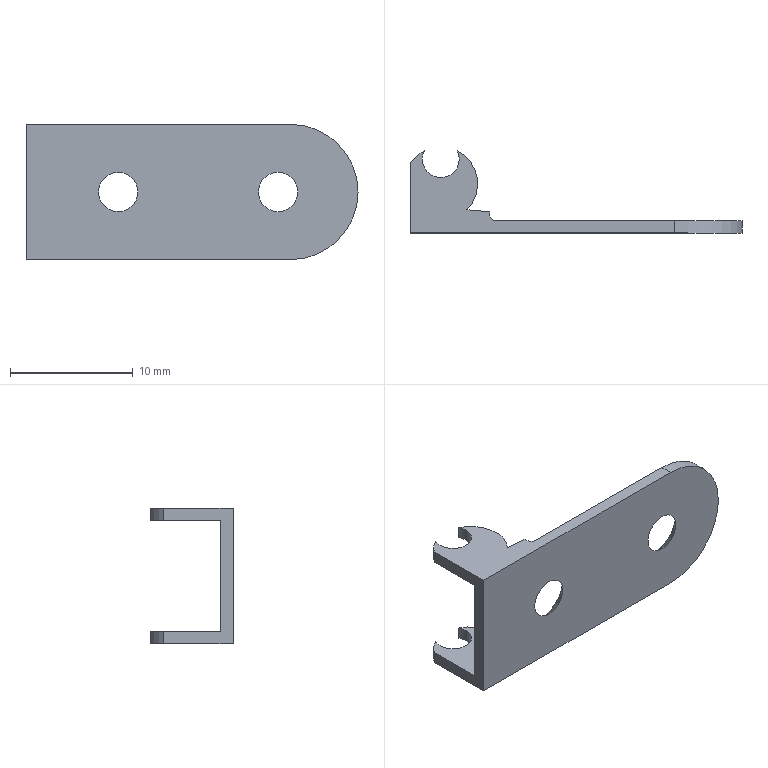Part | SolidWorks | features RefAxis 3, ICE 2, RevCut 2, 3DProfileFeature 1, Extrusion 1 | 1 solid | 28 faces | box 27 x 6.688 x 11 mm | volume 304.183 mm3 | cylinder 13 | plane 11 | cone 4 | commonest cylinder face diameters 3 x6 6 x4 1 x2 11 x1
STEP:
#1=CARTESIAN_POINT('',(20.5,0.,-1.6));
#2=VERTEX_POINT('',#1);
#3=CARTESIAN_POINT('',(20.5,0.,1.6));
#4=VERTEX_POINT('',#3);
#5=CARTESIAN_POINT('',(20.5,0.,0.));
#6=DIRECTION('',(0.,1.,0.));
#7=DIRECTION('',(0.,0.,1.));
#8=AXIS2_PLACEMENT_3D('',#5,#6,#7);
#9=CIRCLE('',#8,1.6);
#10=EDGE_CURVE('',#2,#4,#9,.T.);
#11=ORIENTED_EDGE('',*,*,#10,.F.);
#12=CARTESIAN_POINT('',(20.5,1.,-2.6));
#13=VERTEX_POINT('',#12);
#14=CARTESIAN_POINT('',(20.5,0.,-1.6));
#15=DIRECTION('',(0.,0.7071,-0.7071));
#16=VECTOR('',#15,1000.);
#17=LINE('',#14,#16);
#18=EDGE_CURVE('',#2,#13,#17,.T.);
#19=ORIENTED_EDGE('',*,*,#18,.T.);
#20=CARTESIAN_POINT('',(20.5,1.,2.6));
#21=VERTEX_POINT('',#20);
#22=CARTESIAN_POINT('',(20.5,1.,0.));
#23=DIRECTION('',(0.,1.,0.));
#24=DIRECTION('',(0.,0.,1.));
#25=AXIS2_PLACEMENT_3D('',#22,#23,#24);
#26=CIRCLE('',#25,2.6);
#27=EDGE_CURVE('',#13,#21,#26,.T.);
#28=ORIENTED_EDGE('',*,*,#27,.T.);
#29=CARTESIAN_POINT('',(20.5,0.,1.6));
#30=DIRECTION('',(0.,0.7071,0.7071));
#31=VECTOR('',#30,1000.);
#32=LINE('',#29,#31);
#33=EDGE_CURVE('',#4,#21,#32,.T.);
#34=ORIENTED_EDGE('',*,*,#33,.F.);
#35=EDGE_LOOP('',(#11,#19,#28,#34));
#36=FACE_OUTER_BOUND('',#35,.T.);
#37=CARTESIAN_POINT('',(20.5,0.,0.));
#38=DIRECTION('',(0.,1.,0.));
#39=DIRECTION('',(0.,0.,1.));
#40=AXIS2_PLACEMENT_3D('',#37,#38,#39);
#41=CONICAL_SURFACE('',#40,1.6,0.7854);
#42=ADVANCED_FACE('',(#36),#41,.F.);
#43=CARTESIAN_POINT('',(7.5,0.,-1.6));
#44=VERTEX_POINT('',#43);
#45=CARTESIAN_POINT('',(7.5,0.,1.6));
#46=VERTEX_POINT('',#45);
#47=CARTESIAN_POINT('',(7.5,0.,0.));
#48=DIRECTION('',(0.,1.,0.));
#49=DIRECTION('',(0.,0.,1.));
#50=AXIS2_PLACEMENT_3D('',#47,#48,#49);
#51=CIRCLE('',#50,1.6);
#52=EDGE_CURVE('',#44,#46,#51,.T.);
#53=ORIENTED_EDGE('',*,*,#52,.F.);
#54=CARTESIAN_POINT('',(7.5,1.,-2.6));
#55=VERTEX_POINT('',#54);
#56=CARTESIAN_POINT('',(7.5,0.,-1.6));
#57=DIRECTION('',(0.,0.7071,-0.7071));
#58=VECTOR('',#57,1000.);
#59=LINE('',#56,#58);
#60=EDGE_CURVE('',#44,#55,#59,.T.);
#61=ORIENTED_EDGE('',*,*,#60,.T.);
#62=CARTESIAN_POINT('',(7.5,1.,2.6));
#63=VERTEX_POINT('',#62);
#64=CARTESIAN_POINT('',(7.5,1.,0.));
#65=DIRECTION('',(0.,1.,0.));
#66=DIRECTION('',(0.,0.,1.));
#67=AXIS2_PLACEMENT_3D('',#64,#65,#66);
#68=CIRCLE('',#67,2.6);
#69=EDGE_CURVE('',#55,#63,#68,.T.);
#70=ORIENTED_EDGE('',*,*,#69,.T.);
#71=CARTESIAN_POINT('',(7.5,0.,1.6));
#72=DIRECTION('',(0.,0.7071,0.7071));
#73=VECTOR('',#72,1000.);
#74=LINE('',#71,#73);
#75=EDGE_CURVE('',#46,#63,#74,.T.);
#76=ORIENTED_EDGE('',*,*,#75,.F.);
#77=EDGE_LOOP('',(#53,#61,#70,#76));
#78=FACE_OUTER_BOUND('',#77,.T.);
#79=CARTESIAN_POINT('',(7.5,0.,0.));
#80=DIRECTION('',(0.,1.,0.));
#81=DIRECTION('',(0.,0.,1.));
#82=AXIS2_PLACEMENT_3D('',#79,#80,#81);
#83=CONICAL_SURFACE('',#82,1.6,0.7854);
#84=ADVANCED_FACE('',(#78),#83,.F.);
#85=CARTESIAN_POINT('',(4.,6.,-4.5));
#86=VERTEX_POINT('',#85);
#87=CARTESIAN_POINT('',(1.,6.,-4.5));
#88=VERTEX_POINT('',#87);
#89=CARTESIAN_POINT('',(2.5,6.,-4.5));
#90=DIRECTION('',(0.,0.,-1.));
#91=DIRECTION('',(1.,0.,0.));
#92=AXIS2_PLACEMENT_3D('',#89,#90,#91);
#93=CIRCLE('',#92,1.5);
#94=EDGE_CURVE('',#86,#88,#93,.T.);
#95=ORIENTED_EDGE('',*,*,#94,.F.);
#96=CARTESIAN_POINT('',(4.,6.,-5.5));
#97=VERTEX_POINT('',#96);
#98=CARTESIAN_POINT('',(4.,6.,5.5));
#99=DIRECTION('',(0.,0.,-1.));
#100=VECTOR('',#99,1000.);
#101=LINE('',#98,#100);
#102=EDGE_CURVE('',#86,#97,#101,.T.);
#103=ORIENTED_EDGE('',*,*,#102,.T.);
#104=CARTESIAN_POINT('',(1.,6.,-5.5));
#105=VERTEX_POINT('',#104);
#106=CARTESIAN_POINT('',(2.5,6.,-5.5));
#107=DIRECTION('',(0.,0.,-1.));
#108=DIRECTION('',(-1.,0.,0.));
#109=AXIS2_PLACEMENT_3D('',#106,#107,#108);
#110=CIRCLE('',#109,1.5);
#111=EDGE_CURVE('',#97,#105,#110,.T.);
#112=ORIENTED_EDGE('',*,*,#111,.T.);
#113=CARTESIAN_POINT('',(1.,6.,5.5));
#114=DIRECTION('',(0.,0.,-1.));
#115=VECTOR('',#114,1000.);
#116=LINE('',#113,#115);
#117=EDGE_CURVE('',#88,#105,#116,.T.);
#118=ORIENTED_EDGE('',*,*,#117,.F.);
#119=EDGE_LOOP('',(#95,#103,#112,#118));
#120=FACE_OUTER_BOUND('',#119,.T.);
#121=CARTESIAN_POINT('',(2.5,6.,5.5));
#122=DIRECTION('',(0.,0.,-1.));
#123=DIRECTION('',(-1.,0.,0.));
#124=AXIS2_PLACEMENT_3D('',#121,#122,#123);
#125=CYLINDRICAL_SURFACE('',#124,1.5);
#126=ADVANCED_FACE('',(#120),#125,.F.);
#127=CARTESIAN_POINT('',(1.167,6.688,-4.5));
#128=VERTEX_POINT('',#127);
#129=CARTESIAN_POINT('',(2.5,6.,-4.5));
#130=DIRECTION('',(0.,0.,-1.));
#131=DIRECTION('',(1.,0.,0.));
#132=AXIS2_PLACEMENT_3D('',#129,#130,#131);
#133=CIRCLE('',#132,1.5);
#134=EDGE_CURVE('',#88,#128,#133,.T.);
#135=ORIENTED_EDGE('',*,*,#134,.F.);
#136=ORIENTED_EDGE('',*,*,#117,.T.);
#137=CARTESIAN_POINT('',(1.167,6.688,-5.5));
#138=VERTEX_POINT('',#137);
#139=CARTESIAN_POINT('',(2.5,6.,-5.5));
#140=DIRECTION('',(0.,0.,-1.));
#141=DIRECTION('',(-1.,0.,0.));
#142=AXIS2_PLACEMENT_3D('',#139,#140,#141);
#143=CIRCLE('',#142,1.5);
#144=EDGE_CURVE('',#105,#138,#143,.T.);
#145=ORIENTED_EDGE('',*,*,#144,.T.);
#146=CARTESIAN_POINT('',(1.167,6.688,5.5));
#147=DIRECTION('',(0.,0.,-1.));
#148=VECTOR('',#147,1000.);
#149=LINE('',#146,#148);
#150=EDGE_CURVE('',#128,#138,#149,.T.);
#151=ORIENTED_EDGE('',*,*,#150,.F.);
#152=EDGE_LOOP('',(#135,#136,#145,#151));
#153=FACE_OUTER_BOUND('',#152,.T.);
#154=CARTESIAN_POINT('',(2.5,6.,5.5));
#155=DIRECTION('',(0.,0.,-1.));
#156=DIRECTION('',(-1.,0.,0.));
#157=AXIS2_PLACEMENT_3D('',#154,#155,#156);
#158=CYLINDRICAL_SURFACE('',#157,1.5);
#159=ADVANCED_FACE('',(#153),#158,.F.);
#160=CARTESIAN_POINT('',(4.,6.,5.5));
#161=VERTEX_POINT('',#160);
#162=CARTESIAN_POINT('',(1.,6.,5.5));
#163=VERTEX_POINT('',#162);
#164=CARTESIAN_POINT('',(2.5,6.,5.5));
#165=DIRECTION('',(0.,0.,-1.));
#166=DIRECTION('',(-1.,0.,0.));
#167=AXIS2_PLACEMENT_3D('',#164,#165,#166);
#168=CIRCLE('',#167,1.5);
#169=EDGE_CURVE('',#161,#163,#168,.T.);
#170=ORIENTED_EDGE('',*,*,#169,.F.);
#171=CARTESIAN_POINT('',(4.,6.,4.5));
#172=VERTEX_POINT('',#171);
#173=CARTESIAN_POINT('',(4.,6.,5.5));
#174=DIRECTION('',(0.,0.,-1.));
#175=VECTOR('',#174,1000.);
#176=LINE('',#173,#175);
#177=EDGE_CURVE('',#161,#172,#176,.T.);
#178=ORIENTED_EDGE('',*,*,#177,.T.);
#179=CARTESIAN_POINT('',(1.,6.,4.5));
#180=VERTEX_POINT('',#179);
#181=CARTESIAN_POINT('',(2.5,6.,4.5));
#182=DIRECTION('',(0.,0.,1.));
#183=DIRECTION('',(-1.,0.,0.));
#184=AXIS2_PLACEMENT_3D('',#181,#182,#183);
#185=CIRCLE('',#184,1.5);
#186=EDGE_CURVE('',#180,#172,#185,.T.);
#187=ORIENTED_EDGE('',*,*,#186,.F.);
#188=CARTESIAN_POINT('',(1.,6.,5.5));
#189=DIRECTION('',(0.,0.,-1.));
#190=VECTOR('',#189,1000.);
#191=LINE('',#188,#190);
#192=EDGE_CURVE('',#163,#180,#191,.T.);
#193=ORIENTED_EDGE('',*,*,#192,.F.);
#194=EDGE_LOOP('',(#170,#178,#187,#193));
#195=FACE_OUTER_BOUND('',#194,.T.);
#196=CARTESIAN_POINT('',(2.5,6.,5.5));
#197=DIRECTION('',(0.,0.,-1.));
#198=DIRECTION('',(-1.,0.,0.));
#199=AXIS2_PLACEMENT_3D('',#196,#197,#198);
#200=CYLINDRICAL_SURFACE('',#199,1.5);
#201=ADVANCED_FACE('',(#195),#200,.F.);
#202=CARTESIAN_POINT('',(1.167,6.688,5.5));
#203=VERTEX_POINT('',#202);
#204=CARTESIAN_POINT('',(2.5,6.,5.5));
#205=DIRECTION('',(0.,0.,-1.));
#206=DIRECTION('',(-1.,0.,0.));
#207=AXIS2_PLACEMENT_3D('',#204,#205,#206);
#208=CIRCLE('',#207,1.5);
#209=EDGE_CURVE('',#163,#203,#208,.T.);
#210=ORIENTED_EDGE('',*,*,#209,.F.);
#211=ORIENTED_EDGE('',*,*,#192,.T.);
#212=CARTESIAN_POINT('',(1.167,6.687,4.5));
#213=VERTEX_POINT('',#212);
#214=CARTESIAN_POINT('',(2.5,6.,4.5));
#215=DIRECTION('',(0.,0.,1.));
#216=DIRECTION('',(-1.,0.,0.));
#217=AXIS2_PLACEMENT_3D('',#214,#215,#216);
#218=CIRCLE('',#217,1.5);
#219=EDGE_CURVE('',#213,#180,#218,.T.);
#220=ORIENTED_EDGE('',*,*,#219,.F.);
#221=CARTESIAN_POINT('',(1.167,6.688,5.5));
#222=DIRECTION('',(0.,0.,-1.));
#223=VECTOR('',#222,1000.);
#224=LINE('',#221,#223);
#225=EDGE_CURVE('',#203,#213,#224,.T.);
#226=ORIENTED_EDGE('',*,*,#225,.F.);
#227=EDGE_LOOP('',(#210,#211,#220,#226));
#228=FACE_OUTER_BOUND('',#227,.T.);
#229=CARTESIAN_POINT('',(2.5,6.,5.5));
#230=DIRECTION('',(0.,0.,-1.));
#231=DIRECTION('',(-1.,0.,0.));
#232=AXIS2_PLACEMENT_3D('',#229,#230,#231);
#233=CYLINDRICAL_SURFACE('',#232,1.5);
#234=ADVANCED_FACE('',(#228),#233,.F.);
#235=CARTESIAN_POINT('',(7.5,0.,0.));
#236=DIRECTION('',(0.,1.,0.));
#237=DIRECTION('',(0.,0.,1.));
#238=AXIS2_PLACEMENT_3D('',#235,#236,#237);
#239=CIRCLE('',#238,1.6);
#240=EDGE_CURVE('',#46,#44,#239,.T.);
#241=ORIENTED_EDGE('',*,*,#240,.T.);
#242=ORIENTED_EDGE('',*,*,#52,.T.);
#243=EDGE_LOOP('',(#241,#242));
#244=FACE_BOUND('',#243,.T.);
#245=CARTESIAN_POINT('',(0.,0.,-5.5));
#246=VERTEX_POINT('',#245);
#247=CARTESIAN_POINT('',(21.5,0.,-5.5));
#248=VERTEX_POINT('',#247);
#249=CARTESIAN_POINT('',(0.,0.,-5.5));
#250=DIRECTION('',(1.,0.,0.));
#251=VECTOR('',#250,1000.);
#252=LINE('',#249,#251);
#253=EDGE_CURVE('',#246,#248,#252,.T.);
#254=ORIENTED_EDGE('',*,*,#253,.T.);
#255=CARTESIAN_POINT('',(21.5,0.,5.5));
#256=VERTEX_POINT('',#255);
#257=CARTESIAN_POINT('',(21.5,0.,0.));
#258=DIRECTION('',(0.,1.,0.));
#259=DIRECTION('',(0.,0.,1.));
#260=AXIS2_PLACEMENT_3D('',#257,#258,#259);
#261=CIRCLE('',#260,5.5);
#262=EDGE_CURVE('',#256,#248,#261,.T.);
#263=ORIENTED_EDGE('',*,*,#262,.F.);
#264=CARTESIAN_POINT('',(0.,0.,5.5));
#265=VERTEX_POINT('',#264);
#266=CARTESIAN_POINT('',(0.,0.,5.5));
#267=DIRECTION('',(1.,0.,0.));
#268=VECTOR('',#267,1000.);
#269=LINE('',#266,#268);
#270=EDGE_CURVE('',#265,#256,#269,.T.);
#271=ORIENTED_EDGE('',*,*,#270,.F.);
#272=CARTESIAN_POINT('',(0.,0.,5.5));
#273=DIRECTION('',(0.,0.,-1.));
#274=VECTOR('',#273,1000.);
#275=LINE('',#272,#274);
#276=EDGE_CURVE('',#265,#246,#275,.T.);
#277=ORIENTED_EDGE('',*,*,#276,.T.);
#278=EDGE_LOOP('',(#254,#263,#271,#277));
#279=FACE_OUTER_BOUND('',#278,.T.);
#280=CARTESIAN_POINT('',(20.5,0.,0.));
#281=DIRECTION('',(0.,1.,0.));
#282=DIRECTION('',(0.,0.,1.));
#283=AXIS2_PLACEMENT_3D('',#280,#281,#282);
#284=CIRCLE('',#283,1.6);
#285=EDGE_CURVE('',#4,#2,#284,.T.);
#286=ORIENTED_EDGE('',*,*,#285,.T.);
#287=ORIENTED_EDGE('',*,*,#10,.T.);
#288=EDGE_LOOP('',(#286,#287));
#289=FACE_BOUND('',#288,.T.);
#290=CARTESIAN_POINT('',(0.,0.,5.5));
#291=DIRECTION('',(0.,1.,0.));
#292=DIRECTION('',(0.,0.,1.));
#293=AXIS2_PLACEMENT_3D('',#290,#291,#292);
#294=PLANE('',#293);
#295=ADVANCED_FACE('',(#244,#279,#289),#294,.F.);
#296=CARTESIAN_POINT('',(7.5,1.,0.));
#297=DIRECTION('',(0.,1.,0.));
#298=DIRECTION('',(0.,0.,1.));
#299=AXIS2_PLACEMENT_3D('',#296,#297,#298);
#300=CIRCLE('',#299,2.6);
#301=EDGE_CURVE('',#63,#55,#300,.T.);
#302=ORIENTED_EDGE('',*,*,#301,.F.);
#303=ORIENTED_EDGE('',*,*,#69,.F.);
#304=EDGE_LOOP('',(#302,#303));
#305=FACE_BOUND('',#304,.T.);
#306=CARTESIAN_POINT('',(6.99,1.,-4.5));
#307=VERTEX_POINT('',#306);
#308=CARTESIAN_POINT('',(6.99,1.,-5.5));
#309=VERTEX_POINT('',#308);
#310=CARTESIAN_POINT('',(6.99,1.,5.5));
#311=DIRECTION('',(0.,0.,-1.));
#312=VECTOR('',#311,1000.);
#313=LINE('',#310,#312);
#314=EDGE_CURVE('',#307,#309,#313,.T.);
#315=ORIENTED_EDGE('',*,*,#314,.F.);
#316=CARTESIAN_POINT('',(0.,1.,-4.5));
#317=VERTEX_POINT('',#316);
#318=CARTESIAN_POINT('',(11.,1.,-4.5));
#319=DIRECTION('',(-1.,0.,0.));
#320=VECTOR('',#319,1000.);
#321=LINE('',#318,#320);
#322=EDGE_CURVE('',#307,#317,#321,.T.);
#323=ORIENTED_EDGE('',*,*,#322,.T.);
#324=CARTESIAN_POINT('',(0.,1.,4.5));
#325=VERTEX_POINT('',#324);
#326=CARTESIAN_POINT('',(0.,1.,4.5));
#327=DIRECTION('',(0.,0.,-1.));
#328=VECTOR('',#327,1000.);
#329=LINE('',#326,#328);
#330=EDGE_CURVE('',#325,#317,#329,.T.);
#331=ORIENTED_EDGE('',*,*,#330,.F.);
#332=CARTESIAN_POINT('',(6.99,1.,4.5));
#333=VERTEX_POINT('',#332);
#334=CARTESIAN_POINT('',(11.,1.,4.5));
#335=DIRECTION('',(-1.,0.,0.));
#336=VECTOR('',#335,1000.);
#337=LINE('',#334,#336);
#338=EDGE_CURVE('',#333,#325,#337,.T.);
#339=ORIENTED_EDGE('',*,*,#338,.F.);
#340=CARTESIAN_POINT('',(6.99,1.,5.5));
#341=VERTEX_POINT('',#340);
#342=CARTESIAN_POINT('',(6.99,1.,5.5));
#343=DIRECTION('',(0.,0.,-1.));
#344=VECTOR('',#343,1000.);
#345=LINE('',#342,#344);
#346=EDGE_CURVE('',#341,#333,#345,.T.);
#347=ORIENTED_EDGE('',*,*,#346,.F.);
#348=CARTESIAN_POINT('',(21.5,1.,5.5));
#349=VERTEX_POINT('',#348);
#350=CARTESIAN_POINT('',(27.,1.,5.5));
#351=DIRECTION('',(-1.,0.,0.));
#352=VECTOR('',#351,1000.);
#353=LINE('',#350,#352);
#354=EDGE_CURVE('',#349,#341,#353,.T.);
#355=ORIENTED_EDGE('',*,*,#354,.F.);
#356=CARTESIAN_POINT('',(21.5,1.,-5.5));
#357=VERTEX_POINT('',#356);
#358=CARTESIAN_POINT('',(21.5,1.,0.));
#359=DIRECTION('',(0.,1.,0.));
#360=DIRECTION('',(0.,0.,-1.));
#361=AXIS2_PLACEMENT_3D('',#358,#359,#360);
#362=CIRCLE('',#361,5.5);
#363=EDGE_CURVE('',#349,#357,#362,.T.);
#364=ORIENTED_EDGE('',*,*,#363,.T.);
#365=CARTESIAN_POINT('',(27.,1.,-5.5));
#366=DIRECTION('',(-1.,0.,0.));
#367=VECTOR('',#366,1000.);
#368=LINE('',#365,#367);
#369=EDGE_CURVE('',#357,#309,#368,.T.);
#370=ORIENTED_EDGE('',*,*,#369,.T.);
#371=EDGE_LOOP('',(#315,#323,#331,#339,#347,#355,#364,#370));
#372=FACE_OUTER_BOUND('',#371,.T.);
#373=CARTESIAN_POINT('',(20.5,1.,0.));
#374=DIRECTION('',(0.,1.,0.));
#375=DIRECTION('',(0.,0.,1.));
#376=AXIS2_PLACEMENT_3D('',#373,#374,#375);
#377=CIRCLE('',#376,2.6);
#378=EDGE_CURVE('',#21,#13,#377,.T.);
#379=ORIENTED_EDGE('',*,*,#378,.F.);
#380=ORIENTED_EDGE('',*,*,#27,.F.);
#381=EDGE_LOOP('',(#379,#380));
#382=FACE_BOUND('',#381,.T.);
#383=CARTESIAN_POINT('',(27.,1.,5.5));
#384=DIRECTION('',(0.,-1.,0.));
#385=DIRECTION('',(0.,0.,-1.));
#386=AXIS2_PLACEMENT_3D('',#383,#384,#385);
#387=PLANE('',#386);
#388=ADVANCED_FACE('',(#305,#372,#382),#387,.F.);
#389=CARTESIAN_POINT('',(0.,5.658,4.5));
#390=VERTEX_POINT('',#389);
#391=CARTESIAN_POINT('',(0.,11.,4.5));
#392=DIRECTION('',(0.,-1.,0.));
#393=VECTOR('',#392,1000.);
#394=LINE('',#391,#393);
#395=EDGE_CURVE('',#390,#325,#394,.T.);
#396=ORIENTED_EDGE('',*,*,#395,.T.);
#397=ORIENTED_EDGE('',*,*,#330,.T.);
#398=CARTESIAN_POINT('',(0.,5.658,-4.5));
#399=VERTEX_POINT('',#398);
#400=CARTESIAN_POINT('',(0.,1.,-4.5));
#401=DIRECTION('',(0.,1.,0.));
#402=VECTOR('',#401,1000.);
#403=LINE('',#400,#402);
#404=EDGE_CURVE('',#317,#399,#403,.T.);
#405=ORIENTED_EDGE('',*,*,#404,.T.);
#406=CARTESIAN_POINT('',(0.,5.658,-5.5));
#407=VERTEX_POINT('',#406);
#408=CARTESIAN_POINT('',(0.,5.658,5.5));
#409=DIRECTION('',(0.,0.,-1.));
#410=VECTOR('',#409,1000.);
#411=LINE('',#408,#410);
#412=EDGE_CURVE('',#399,#407,#411,.T.);
#413=ORIENTED_EDGE('',*,*,#412,.T.);
#414=CARTESIAN_POINT('',(0.,5.658,-5.5));
#415=DIRECTION('',(0.,-1.,0.));
#416=VECTOR('',#415,1000.);
#417=LINE('',#414,#416);
#418=EDGE_CURVE('',#407,#246,#417,.T.);
#419=ORIENTED_EDGE('',*,*,#418,.T.);
#420=ORIENTED_EDGE('',*,*,#276,.F.);
#421=CARTESIAN_POINT('',(0.,5.658,5.5));
#422=VERTEX_POINT('',#421);
#423=CARTESIAN_POINT('',(0.,5.658,5.5));
#424=DIRECTION('',(0.,-1.,0.));
#425=VECTOR('',#424,1000.);
#426=LINE('',#423,#425);
#427=EDGE_CURVE('',#422,#265,#426,.T.);
#428=ORIENTED_EDGE('',*,*,#427,.F.);
#429=CARTESIAN_POINT('',(0.,5.658,5.5));
#430=DIRECTION('',(0.,0.,-1.));
#431=VECTOR('',#430,1000.);
#432=LINE('',#429,#431);
#433=EDGE_CURVE('',#422,#390,#432,.T.);
#434=ORIENTED_EDGE('',*,*,#433,.T.);
#435=EDGE_LOOP('',(#396,#397,#405,#413,#419,#420,#428,#434));
#436=FACE_OUTER_BOUND('',#435,.T.);
#437=CARTESIAN_POINT('',(0.,5.658,5.5));
#438=DIRECTION('',(1.,0.,0.));
#439=DIRECTION('',(0.,0.,-1.));
#440=AXIS2_PLACEMENT_3D('',#437,#438,#439);
#441=PLANE('',#440);
#442=ADVANCED_FACE('',(#436),#441,.F.);
#443=CARTESIAN_POINT('',(6.49,1.5,4.5));
#444=VERTEX_POINT('',#443);
#445=CARTESIAN_POINT('',(6.99,1.5,4.5));
#446=DIRECTION('',(0.,0.,1.));
#447=DIRECTION('',(-1.,0.,0.));
#448=AXIS2_PLACEMENT_3D('',#445,#446,#447);
#449=CIRCLE('',#448,0.5);
#450=EDGE_CURVE('',#444,#333,#449,.T.);
#451=ORIENTED_EDGE('',*,*,#450,.F.);
#452=CARTESIAN_POINT('',(6.49,1.5,5.5));
#453=VERTEX_POINT('',#452);
#454=CARTESIAN_POINT('',(6.49,1.5,5.5));
#455=DIRECTION('',(0.,0.,-1.));
#456=VECTOR('',#455,1000.);
#457=LINE('',#454,#456);
#458=EDGE_CURVE('',#453,#444,#457,.T.);
#459=ORIENTED_EDGE('',*,*,#458,.F.);
#460=CARTESIAN_POINT('',(6.99,1.5,5.5));
#461=DIRECTION('',(0.,0.,-1.));
#462=DIRECTION('',(-1.,0.,0.));
#463=AXIS2_PLACEMENT_3D('',#460,#461,#462);
#464=CIRCLE('',#463,0.5);
#465=EDGE_CURVE('',#341,#453,#464,.T.);
#466=ORIENTED_EDGE('',*,*,#465,.F.);
#467=ORIENTED_EDGE('',*,*,#346,.T.);
#468=EDGE_LOOP('',(#451,#459,#466,#467));
#469=FACE_OUTER_BOUND('',#468,.T.);
#470=CARTESIAN_POINT('',(6.99,1.5,5.5));
#471=DIRECTION('',(0.,0.,-1.));
#472=DIRECTION('',(-1.,0.,0.));
#473=AXIS2_PLACEMENT_3D('',#470,#471,#472);
#474=CYLINDRICAL_SURFACE('',#473,0.5);
#475=ADVANCED_FACE('',(#469),#474,.F.);
#476=CARTESIAN_POINT('',(6.49,1.5,-4.5));
#477=VERTEX_POINT('',#476);
#478=CARTESIAN_POINT('',(6.99,1.5,-4.5));
#479=DIRECTION('',(0.,0.,-1.));
#480=DIRECTION('',(1.,0.,0.));
#481=AXIS2_PLACEMENT_3D('',#478,#479,#480);
#482=CIRCLE('',#481,0.5);
#483=EDGE_CURVE('',#307,#477,#482,.T.);
#484=ORIENTED_EDGE('',*,*,#483,.F.);
#485=ORIENTED_EDGE('',*,*,#314,.T.);
#486=CARTESIAN_POINT('',(6.49,1.5,-5.5));
#487=VERTEX_POINT('',#486);
#488=CARTESIAN_POINT('',(6.99,1.5,-5.5));
#489=DIRECTION('',(0.,0.,-1.));
#490=DIRECTION('',(-1.,0.,0.));
#491=AXIS2_PLACEMENT_3D('',#488,#489,#490);
#492=CIRCLE('',#491,0.5);
#493=EDGE_CURVE('',#309,#487,#492,.T.);
#494=ORIENTED_EDGE('',*,*,#493,.T.);
#495=CARTESIAN_POINT('',(6.49,1.5,5.5));
#496=DIRECTION('',(0.,0.,-1.));
#497=VECTOR('',#496,1000.);
#498=LINE('',#495,#497);
#499=EDGE_CURVE('',#477,#487,#498,.T.);
#500=ORIENTED_EDGE('',*,*,#499,.F.);
#501=EDGE_LOOP('',(#484,#485,#494,#500));
#502=FACE_OUTER_BOUND('',#501,.T.);
#503=CARTESIAN_POINT('',(6.99,1.5,5.5));
#504=DIRECTION('',(0.,0.,-1.));
#505=DIRECTION('',(-1.,0.,0.));
#506=AXIS2_PLACEMENT_3D('',#503,#504,#505);
#507=CYLINDRICAL_SURFACE('',#506,0.5);
#508=ADVANCED_FACE('',(#502),#507,.F.);
#509=CARTESIAN_POINT('',(6.49,1.725,4.5));
#510=VERTEX_POINT('',#509);
#511=CARTESIAN_POINT('',(6.49,1.5,4.5));
#512=DIRECTION('',(0.,-1.,0.));
#513=VECTOR('',#512,1000.);
#514=LINE('',#511,#513);
#515=EDGE_CURVE('',#510,#444,#514,.T.);
#516=ORIENTED_EDGE('',*,*,#515,.F.);
#517=CARTESIAN_POINT('',(6.49,1.725,5.5));
#518=VERTEX_POINT('',#517);
#519=CARTESIAN_POINT('',(6.49,1.725,5.5));
#520=DIRECTION('',(0.,0.,-1.));
#521=VECTOR('',#520,1000.);
#522=LINE('',#519,#521);
#523=EDGE_CURVE('',#518,#510,#522,.T.);
#524=ORIENTED_EDGE('',*,*,#523,.F.);
#525=CARTESIAN_POINT('',(6.49,1.5,5.5));
#526=DIRECTION('',(0.,1.,0.));
#527=VECTOR('',#526,1000.);
#528=LINE('',#525,#527);
#529=EDGE_CURVE('',#453,#518,#528,.T.);
#530=ORIENTED_EDGE('',*,*,#529,.F.);
#531=ORIENTED_EDGE('',*,*,#458,.T.);
#532=EDGE_LOOP('',(#516,#524,#530,#531));
#533=FACE_OUTER_BOUND('',#532,.T.);
#534=CARTESIAN_POINT('',(6.49,1.5,5.5));
#535=DIRECTION('',(-1.,0.,0.));
#536=DIRECTION('',(0.,0.,1.));
#537=AXIS2_PLACEMENT_3D('',#534,#535,#536);
#538=PLANE('',#537);
#539=ADVANCED_FACE('',(#533),#538,.F.);
#540=CARTESIAN_POINT('',(6.49,1.725,-4.5));
#541=VERTEX_POINT('',#540);
#542=CARTESIAN_POINT('',(6.49,1.5,-4.5));
#543=DIRECTION('',(0.,1.,0.));
#544=VECTOR('',#543,1000.);
#545=LINE('',#542,#544);
#546=EDGE_CURVE('',#477,#541,#545,.T.);
#547=ORIENTED_EDGE('',*,*,#546,.F.);
#548=ORIENTED_EDGE('',*,*,#499,.T.);
#549=CARTESIAN_POINT('',(6.49,1.725,-5.5));
#550=VERTEX_POINT('',#549);
#551=CARTESIAN_POINT('',(6.49,1.5,-5.5));
#552=DIRECTION('',(0.,1.,0.));
#553=VECTOR('',#552,1000.);
#554=LINE('',#551,#553);
#555=EDGE_CURVE('',#487,#550,#554,.T.);
#556=ORIENTED_EDGE('',*,*,#555,.T.);
#557=CARTESIAN_POINT('',(6.49,1.725,5.5));
#558=DIRECTION('',(0.,0.,-1.));
#559=VECTOR('',#558,1000.);
#560=LINE('',#557,#559);
#561=EDGE_CURVE('',#541,#550,#560,.T.);
#562=ORIENTED_EDGE('',*,*,#561,.F.);
#563=EDGE_LOOP('',(#547,#548,#556,#562));
#564=FACE_OUTER_BOUND('',#563,.T.);
#565=CARTESIAN_POINT('',(6.49,1.5,5.5));
#566=DIRECTION('',(-1.,0.,0.));
#567=DIRECTION('',(0.,0.,1.));
#568=AXIS2_PLACEMENT_3D('',#565,#566,#567);
#569=PLANE('',#568);
#570=ADVANCED_FACE('',(#564),#569,.F.);
#571=CARTESIAN_POINT('',(4.63,1.887,4.5));
#572=VERTEX_POINT('',#571);
#573=CARTESIAN_POINT('',(6.49,1.725,4.5));
#574=DIRECTION('',(0.9962,-0.08716,0.));
#575=VECTOR('',#574,1000.);
#576=LINE('',#573,#575);
#577=EDGE_CURVE('',#572,#510,#576,.T.);
#578=ORIENTED_EDGE('',*,*,#577,.F.);
#579=CARTESIAN_POINT('',(4.63,1.887,5.5));
#580=VERTEX_POINT('',#579);
#581=CARTESIAN_POINT('',(4.63,1.887,5.5));
#582=DIRECTION('',(0.,0.,-1.));
#583=VECTOR('',#582,1000.);
#584=LINE('',#581,#583);
#585=EDGE_CURVE('',#580,#572,#584,.T.);
#586=ORIENTED_EDGE('',*,*,#585,.F.);
#587=CARTESIAN_POINT('',(6.49,1.725,5.5));
#588=DIRECTION('',(-0.9962,0.08716,0.));
#589=VECTOR('',#588,1000.);
#590=LINE('',#587,#589);
#591=EDGE_CURVE('',#518,#580,#590,.T.);
#592=ORIENTED_EDGE('',*,*,#591,.F.);
#593=ORIENTED_EDGE('',*,*,#523,.T.);
#594=EDGE_LOOP('',(#578,#586,#592,#593));
#595=FACE_OUTER_BOUND('',#594,.T.);
#596=CARTESIAN_POINT('',(6.49,1.725,5.5));
#597=DIRECTION('',(-0.08716,-0.9962,0.));
#598=DIRECTION('',(0.9962,-0.08716,0.));
#599=AXIS2_PLACEMENT_3D('',#596,#597,#598);
#600=PLANE('',#599);
#601=ADVANCED_FACE('',(#595),#600,.F.);
#602=CARTESIAN_POINT('',(4.63,1.887,-4.5));
#603=VERTEX_POINT('',#602);
#604=CARTESIAN_POINT('',(6.49,1.725,-4.5));
#605=DIRECTION('',(-0.9962,0.08716,0.));
#606=VECTOR('',#605,1000.);
#607=LINE('',#604,#606);
#608=EDGE_CURVE('',#541,#603,#607,.T.);
#609=ORIENTED_EDGE('',*,*,#608,.F.);
#610=ORIENTED_EDGE('',*,*,#561,.T.);
#611=CARTESIAN_POINT('',(4.63,1.887,-5.5));
#612=VERTEX_POINT('',#611);
#613=CARTESIAN_POINT('',(6.49,1.725,-5.5));
#614=DIRECTION('',(-0.9962,0.08716,0.));
#615=VECTOR('',#614,1000.);
#616=LINE('',#613,#615);
#617=EDGE_CURVE('',#550,#612,#616,.T.);
#618=ORIENTED_EDGE('',*,*,#617,.T.);
#619=CARTESIAN_POINT('',(4.63,1.887,5.5));
#620=DIRECTION('',(0.,0.,-1.));
#621=VECTOR('',#620,1000.);
#622=LINE('',#619,#621);
#623=EDGE_CURVE('',#603,#612,#622,.T.);
#624=ORIENTED_EDGE('',*,*,#623,.F.);
#625=EDGE_LOOP('',(#609,#610,#618,#624));
#626=FACE_OUTER_BOUND('',#625,.T.);
#627=CARTESIAN_POINT('',(6.49,1.725,5.5));
#628=DIRECTION('',(-0.08716,-0.9962,0.));
#629=DIRECTION('',(0.9962,-0.08716,0.));
#630=AXIS2_PLACEMENT_3D('',#627,#628,#629);
#631=PLANE('',#630);
#632=ADVANCED_FACE('',(#626),#631,.F.);
#633=CARTESIAN_POINT('',(3.833,6.687,4.5));
#634=VERTEX_POINT('',#633);
#635=CARTESIAN_POINT('',(2.5,4.,4.5));
#636=DIRECTION('',(0.,0.,-1.));
#637=DIRECTION('',(-1.,0.,0.));
#638=AXIS2_PLACEMENT_3D('',#635,#636,#637);
#639=CIRCLE('',#638,3.);
#640=EDGE_CURVE('',#634,#572,#639,.T.);
#641=ORIENTED_EDGE('',*,*,#640,.F.);
#642=CARTESIAN_POINT('',(3.833,6.687,5.5));
#643=VERTEX_POINT('',#642);
#644=CARTESIAN_POINT('',(3.833,6.687,5.5));
#645=DIRECTION('',(0.,0.,-1.));
#646=VECTOR('',#645,1000.);
#647=LINE('',#644,#646);
#648=EDGE_CURVE('',#643,#634,#647,.T.);
#649=ORIENTED_EDGE('',*,*,#648,.F.);
#650=CARTESIAN_POINT('',(2.5,4.,5.5));
#651=DIRECTION('',(0.,0.,1.));
#652=DIRECTION('',(1.,0.,0.));
#653=AXIS2_PLACEMENT_3D('',#650,#651,#652);
#654=CIRCLE('',#653,3.);
#655=EDGE_CURVE('',#580,#643,#654,.T.);
#656=ORIENTED_EDGE('',*,*,#655,.F.);
#657=ORIENTED_EDGE('',*,*,#585,.T.);
#658=EDGE_LOOP('',(#641,#649,#656,#657));
#659=FACE_OUTER_BOUND('',#658,.T.);
#660=CARTESIAN_POINT('',(2.5,4.,5.5));
#661=DIRECTION('',(0.,0.,-1.));
#662=DIRECTION('',(-1.,0.,0.));
#663=AXIS2_PLACEMENT_3D('',#660,#661,#662);
#664=CYLINDRICAL_SURFACE('',#663,3.);
#665=ADVANCED_FACE('',(#659),#664,.T.);
#666=CARTESIAN_POINT('',(3.833,6.687,-4.5));
#667=VERTEX_POINT('',#666);
#668=CARTESIAN_POINT('',(2.5,4.,-4.5));
#669=DIRECTION('',(0.,0.,1.));
#670=DIRECTION('',(1.,0.,0.));
#671=AXIS2_PLACEMENT_3D('',#668,#669,#670);
#672=CIRCLE('',#671,3.);
#673=EDGE_CURVE('',#603,#667,#672,.T.);
#674=ORIENTED_EDGE('',*,*,#673,.F.);
#675=ORIENTED_EDGE('',*,*,#623,.T.);
#676=CARTESIAN_POINT('',(3.833,6.687,-5.5));
#677=VERTEX_POINT('',#676);
#678=CARTESIAN_POINT('',(2.5,4.,-5.5));
#679=DIRECTION('',(0.,0.,1.));
#680=DIRECTION('',(1.,0.,0.));
#681=AXIS2_PLACEMENT_3D('',#678,#679,#680);
#682=CIRCLE('',#681,3.);
#683=EDGE_CURVE('',#612,#677,#682,.T.);
#684=ORIENTED_EDGE('',*,*,#683,.T.);
#685=CARTESIAN_POINT('',(3.833,6.687,5.5));
#686=DIRECTION('',(0.,0.,-1.));
#687=VECTOR('',#686,1000.);
#688=LINE('',#685,#687);
#689=EDGE_CURVE('',#667,#677,#688,.T.);
#690=ORIENTED_EDGE('',*,*,#689,.F.);
#691=EDGE_LOOP('',(#674,#675,#684,#690));
#692=FACE_OUTER_BOUND('',#691,.T.);
#693=CARTESIAN_POINT('',(2.5,4.,5.5));
#694=DIRECTION('',(0.,0.,-1.));
#695=DIRECTION('',(-1.,0.,0.));
#696=AXIS2_PLACEMENT_3D('',#693,#694,#695);
#697=CYLINDRICAL_SURFACE('',#696,3.);
#698=ADVANCED_FACE('',(#692),#697,.T.);
#699=ORIENTED_EDGE('',*,*,#177,.F.);
#700=CARTESIAN_POINT('',(2.5,6.,5.5));
#701=DIRECTION('',(0.,0.,-1.));
#702=DIRECTION('',(-1.,0.,0.));
#703=AXIS2_PLACEMENT_3D('',#700,#701,#702);
#704=CIRCLE('',#703,1.5);
#705=EDGE_CURVE('',#643,#161,#704,.T.);
#706=ORIENTED_EDGE('',*,*,#705,.F.);
#707=ORIENTED_EDGE('',*,*,#648,.T.);
#708=CARTESIAN_POINT('',(2.5,6.,4.5));
#709=DIRECTION('',(0.,0.,1.));
#710=DIRECTION('',(-1.,0.,0.));
#711=AXIS2_PLACEMENT_3D('',#708,#709,#710);
#712=CIRCLE('',#711,1.5);
#713=EDGE_CURVE('',#172,#634,#712,.T.);
#714=ORIENTED_EDGE('',*,*,#713,.F.);
#715=EDGE_LOOP('',(#699,#706,#707,#714));
#716=FACE_OUTER_BOUND('',#715,.T.);
#717=CARTESIAN_POINT('',(2.5,6.,5.5));
#718=DIRECTION('',(0.,0.,-1.));
#719=DIRECTION('',(-1.,0.,0.));
#720=AXIS2_PLACEMENT_3D('',#717,#718,#719);
#721=CYLINDRICAL_SURFACE('',#720,1.5);
#722=ADVANCED_FACE('',(#716),#721,.F.);
#723=ORIENTED_EDGE('',*,*,#102,.F.);
#724=CARTESIAN_POINT('',(2.5,6.,-4.5));
#725=DIRECTION('',(0.,0.,-1.));
#726=DIRECTION('',(1.,0.,0.));
#727=AXIS2_PLACEMENT_3D('',#724,#725,#726);
#728=CIRCLE('',#727,1.5);
#729=EDGE_CURVE('',#667,#86,#728,.T.);
#730=ORIENTED_EDGE('',*,*,#729,.F.);
#731=ORIENTED_EDGE('',*,*,#689,.T.);
#732=CARTESIAN_POINT('',(2.5,6.,-5.5));
#733=DIRECTION('',(0.,0.,-1.));
#734=DIRECTION('',(-1.,0.,0.));
#735=AXIS2_PLACEMENT_3D('',#732,#733,#734);
#736=CIRCLE('',#735,1.5);
#737=EDGE_CURVE('',#677,#97,#736,.T.);
#738=ORIENTED_EDGE('',*,*,#737,.T.);
#739=EDGE_LOOP('',(#723,#730,#731,#738));
#740=FACE_OUTER_BOUND('',#739,.T.);
#741=CARTESIAN_POINT('',(2.5,6.,5.5));
#742=DIRECTION('',(0.,0.,-1.));
#743=DIRECTION('',(-1.,0.,0.));
#744=AXIS2_PLACEMENT_3D('',#741,#742,#743);
#745=CYLINDRICAL_SURFACE('',#744,1.5);
#746=ADVANCED_FACE('',(#740),#745,.F.);
#747=CARTESIAN_POINT('',(2.5,4.,4.5));
#748=DIRECTION('',(0.,0.,-1.));
#749=DIRECTION('',(-1.,0.,0.));
#750=AXIS2_PLACEMENT_3D('',#747,#748,#749);
#751=CIRCLE('',#750,3.);
#752=EDGE_CURVE('',#390,#213,#751,.T.);
#753=ORIENTED_EDGE('',*,*,#752,.F.);
#754=ORIENTED_EDGE('',*,*,#433,.F.);
#755=CARTESIAN_POINT('',(2.5,4.,5.5));
#756=DIRECTION('',(0.,0.,1.));
#757=DIRECTION('',(1.,0.,0.));
#758=AXIS2_PLACEMENT_3D('',#755,#756,#757);
#759=CIRCLE('',#758,3.);
#760=EDGE_CURVE('',#203,#422,#759,.T.);
#761=ORIENTED_EDGE('',*,*,#760,.F.);
#762=ORIENTED_EDGE('',*,*,#225,.T.);
#763=EDGE_LOOP('',(#753,#754,#761,#762));
#764=FACE_OUTER_BOUND('',#763,.T.);
#765=CARTESIAN_POINT('',(2.5,4.,5.5));
#766=DIRECTION('',(0.,0.,-1.));
#767=DIRECTION('',(-1.,0.,0.));
#768=AXIS2_PLACEMENT_3D('',#765,#766,#767);
#769=CYLINDRICAL_SURFACE('',#768,3.);
#770=ADVANCED_FACE('',(#764),#769,.T.);
#771=CARTESIAN_POINT('',(2.5,4.,-4.5));
#772=DIRECTION('',(0.,0.,1.));
#773=DIRECTION('',(1.,0.,0.));
#774=AXIS2_PLACEMENT_3D('',#771,#772,#773);
#775=CIRCLE('',#774,3.);
#776=EDGE_CURVE('',#128,#399,#775,.T.);
#777=ORIENTED_EDGE('',*,*,#776,.F.);
#778=ORIENTED_EDGE('',*,*,#150,.T.);
#779=CARTESIAN_POINT('',(2.5,4.,-5.5));
#780=DIRECTION('',(0.,0.,1.));
#781=DIRECTION('',(1.,0.,0.));
#782=AXIS2_PLACEMENT_3D('',#779,#780,#781);
#783=CIRCLE('',#782,3.);
#784=EDGE_CURVE('',#138,#407,#783,.T.);
#785=ORIENTED_EDGE('',*,*,#784,.T.);
#786=ORIENTED_EDGE('',*,*,#412,.F.);
#787=EDGE_LOOP('',(#777,#778,#785,#786));
#788=FACE_OUTER_BOUND('',#787,.T.);
#789=CARTESIAN_POINT('',(2.5,4.,5.5));
#790=DIRECTION('',(0.,0.,-1.));
#791=DIRECTION('',(-1.,0.,0.));
#792=AXIS2_PLACEMENT_3D('',#789,#790,#791);
#793=CYLINDRICAL_SURFACE('',#792,3.);
#794=ADVANCED_FACE('',(#788),#793,.T.);
#795=ORIENTED_EDGE('',*,*,#270,.T.);
#796=CARTESIAN_POINT('',(21.5,11.,5.5));
#797=DIRECTION('',(0.,-1.,0.));
#798=VECTOR('',#797,1000.);
#799=LINE('',#796,#798);
#800=EDGE_CURVE('',#349,#256,#799,.T.);
#801=ORIENTED_EDGE('',*,*,#800,.F.);
#802=ORIENTED_EDGE('',*,*,#354,.T.);
#803=ORIENTED_EDGE('',*,*,#465,.T.);
#804=ORIENTED_EDGE('',*,*,#529,.T.);
#805=ORIENTED_EDGE('',*,*,#591,.T.);
#806=ORIENTED_EDGE('',*,*,#655,.T.);
#807=ORIENTED_EDGE('',*,*,#705,.T.);
#808=ORIENTED_EDGE('',*,*,#169,.T.);
#809=ORIENTED_EDGE('',*,*,#209,.T.);
#810=ORIENTED_EDGE('',*,*,#760,.T.);
#811=ORIENTED_EDGE('',*,*,#427,.T.);
#812=EDGE_LOOP('',(#795,#801,#802,#803,#804,#805,#806,#807,#808,#809,#810,#811));
#813=FACE_OUTER_BOUND('',#812,.T.);
#814=CARTESIAN_POINT('',(6.99,1.5,5.5));
#815=DIRECTION('',(0.,0.,-1.));
#816=DIRECTION('',(-1.,0.,0.));
#817=AXIS2_PLACEMENT_3D('',#814,#815,#816);
#818=PLANE('',#817);
#819=ADVANCED_FACE('',(#813),#818,.F.);
#820=CARTESIAN_POINT('',(21.5,11.,-5.5));
#821=DIRECTION('',(0.,1.,0.));
#822=VECTOR('',#821,1000.);
#823=LINE('',#820,#822);
#824=EDGE_CURVE('',#248,#357,#823,.T.);
#825=ORIENTED_EDGE('',*,*,#824,.F.);
#826=ORIENTED_EDGE('',*,*,#253,.F.);
#827=ORIENTED_EDGE('',*,*,#418,.F.);
#828=ORIENTED_EDGE('',*,*,#784,.F.);
#829=ORIENTED_EDGE('',*,*,#144,.F.);
#830=ORIENTED_EDGE('',*,*,#111,.F.);
#831=ORIENTED_EDGE('',*,*,#737,.F.);
#832=ORIENTED_EDGE('',*,*,#683,.F.);
#833=ORIENTED_EDGE('',*,*,#617,.F.);
#834=ORIENTED_EDGE('',*,*,#555,.F.);
#835=ORIENTED_EDGE('',*,*,#493,.F.);
#836=ORIENTED_EDGE('',*,*,#369,.F.);
#837=EDGE_LOOP('',(#825,#826,#827,#828,#829,#830,#831,#832,#833,#834,#835,#836));
#838=FACE_OUTER_BOUND('',#837,.T.);
#839=CARTESIAN_POINT('',(6.99,1.5,-5.5));
#840=DIRECTION('',(0.,0.,-1.));
#841=DIRECTION('',(-1.,0.,0.));
#842=AXIS2_PLACEMENT_3D('',#839,#840,#841);
#843=PLANE('',#842);
#844=ADVANCED_FACE('',(#838),#843,.T.);
#845=ORIENTED_EDGE('',*,*,#262,.T.);
#846=ORIENTED_EDGE('',*,*,#824,.T.);
#847=ORIENTED_EDGE('',*,*,#363,.F.);
#848=ORIENTED_EDGE('',*,*,#800,.T.);
#849=EDGE_LOOP('',(#845,#846,#847,#848));
#850=FACE_OUTER_BOUND('',#849,.T.);
#851=CARTESIAN_POINT('',(21.5,11.,0.));
#852=DIRECTION('',(0.,-1.,0.));
#853=DIRECTION('',(0.,0.,-1.));
#854=AXIS2_PLACEMENT_3D('',#851,#852,#853);
#855=CYLINDRICAL_SURFACE('',#854,5.5);
#856=ADVANCED_FACE('',(#850),#855,.T.);
#857=ORIENTED_EDGE('',*,*,#450,.T.);
#858=ORIENTED_EDGE('',*,*,#338,.T.);
#859=ORIENTED_EDGE('',*,*,#395,.F.);
#860=ORIENTED_EDGE('',*,*,#752,.T.);
#861=ORIENTED_EDGE('',*,*,#219,.T.);
#862=ORIENTED_EDGE('',*,*,#186,.T.);
#863=ORIENTED_EDGE('',*,*,#713,.T.);
#864=ORIENTED_EDGE('',*,*,#640,.T.);
#865=ORIENTED_EDGE('',*,*,#577,.T.);
#866=ORIENTED_EDGE('',*,*,#515,.T.);
#867=EDGE_LOOP('',(#857,#858,#859,#860,#861,#862,#863,#864,#865,#866));
#868=FACE_OUTER_BOUND('',#867,.T.);
#869=CARTESIAN_POINT('',(11.,11.,4.5));
#870=DIRECTION('',(0.,0.,-1.));
#871=DIRECTION('',(-1.,0.,0.));
#872=AXIS2_PLACEMENT_3D('',#869,#870,#871);
#873=PLANE('',#872);
#874=ADVANCED_FACE('',(#868),#873,.T.);
#875=ORIENTED_EDGE('',*,*,#483,.T.);
#876=ORIENTED_EDGE('',*,*,#546,.T.);
#877=ORIENTED_EDGE('',*,*,#608,.T.);
#878=ORIENTED_EDGE('',*,*,#673,.T.);
#879=ORIENTED_EDGE('',*,*,#729,.T.);
#880=ORIENTED_EDGE('',*,*,#94,.T.);
#881=ORIENTED_EDGE('',*,*,#134,.T.);
#882=ORIENTED_EDGE('',*,*,#776,.T.);
#883=ORIENTED_EDGE('',*,*,#404,.F.);
#884=ORIENTED_EDGE('',*,*,#322,.F.);
#885=EDGE_LOOP('',(#875,#876,#877,#878,#879,#880,#881,#882,#883,#884));
#886=FACE_OUTER_BOUND('',#885,.T.);
#887=CARTESIAN_POINT('',(11.,1.,-4.5));
#888=DIRECTION('',(0.,0.,1.));
#889=DIRECTION('',(1.,0.,0.));
#890=AXIS2_PLACEMENT_3D('',#887,#888,#889);
#891=PLANE('',#890);
#892=ADVANCED_FACE('',(#886),#891,.T.);
#893=ORIENTED_EDGE('',*,*,#60,.F.);
#894=ORIENTED_EDGE('',*,*,#240,.F.);
#895=ORIENTED_EDGE('',*,*,#75,.T.);
#896=ORIENTED_EDGE('',*,*,#301,.T.);
#897=EDGE_LOOP('',(#893,#894,#895,#896));
#898=FACE_OUTER_BOUND('',#897,.T.);
#899=CARTESIAN_POINT('',(7.5,0.,0.));
#900=DIRECTION('',(0.,1.,0.));
#901=DIRECTION('',(0.,0.,1.));
#902=AXIS2_PLACEMENT_3D('',#899,#900,#901);
#903=CONICAL_SURFACE('',#902,1.6,0.7854);
#904=ADVANCED_FACE('',(#898),#903,.F.);
#905=ORIENTED_EDGE('',*,*,#18,.F.);
#906=ORIENTED_EDGE('',*,*,#285,.F.);
#907=ORIENTED_EDGE('',*,*,#33,.T.);
#908=ORIENTED_EDGE('',*,*,#378,.T.);
#909=EDGE_LOOP('',(#905,#906,#907,#908));
#910=FACE_OUTER_BOUND('',#909,.T.);
#911=CARTESIAN_POINT('',(20.5,0.,0.));
#912=DIRECTION('',(0.,1.,0.));
#913=DIRECTION('',(0.,0.,1.));
#914=AXIS2_PLACEMENT_3D('',#911,#912,#913);
#915=CONICAL_SURFACE('',#914,1.6,0.7854);
#916=ADVANCED_FACE('',(#910),#915,.F.);
#917=CLOSED_SHELL('',(#42,#84,#126,#159,#201,#234,#295,#388,#442,#475,#508,#539,#570,#601,#632,#665,#698,#722,#746,#770,#794,#819,#844,#856,#874,#892,#904,#916));
#918=MANIFOLD_SOLID_BREP('',#917);
#919=CARTESIAN_POINT('',(0.,0.,0.));
#920=DIRECTION('',(0.,0.,1.));
#921=DIRECTION('',(1.,0.,0.));
#922=AXIS2_PLACEMENT_3D('',#919,#920,#921);
#923=(LENGTH_UNIT()NAMED_UNIT(*)SI_UNIT(.MILLI.,.METRE.));
#924=UNCERTAINTY_MEASURE_WITH_UNIT(LENGTH_MEASURE(0.00001),#923,'','');
#925=(NAMED_UNIT(*)PLANE_ANGLE_UNIT()SI_UNIT($,.RADIAN.));
#926=(NAMED_UNIT(*)SI_UNIT($,.STERADIAN.)SOLID_ANGLE_UNIT());
#927=(GEOMETRIC_REPRESENTATION_CONTEXT(3)GLOBAL_UNCERTAINTY_ASSIGNED_CONTEXT((#924))GLOBAL_UNIT_ASSIGNED_CONTEXT((#923,#925,#926))REPRESENTATION_CONTEXT('',''));
#928=ADVANCED_BREP_SHAPE_REPRESENTATION('',(#918,#922),#927);